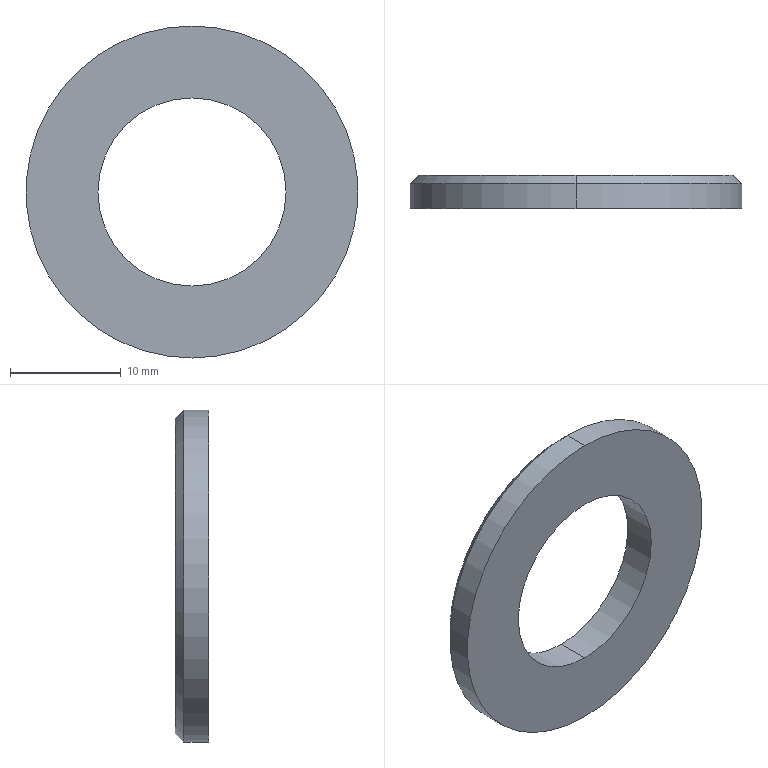Part | STEP file | Flat Washer GB/T97.2-1985 Chamfered Type Grade A 16x3 | 1 solid | 8 faces | box 30 x 3 x 30 mm | volume 1414 mm3 | cylinder 4 | cone 2 | plane 2 | commonest cylinder face diameters 17 x2 30 x2
STEP:
#1=CARTESIAN_POINT('',(0.,0.,0.));
#2=DIRECTION('',(0.,0.,1.));
#3=DIRECTION('',(1.,0.,0.));
#4=AXIS2_PLACEMENT_3D('',#1,#2,#3);
#5=CARTESIAN_POINT('',(0.,10.895,-15.));
#6=VERTEX_POINT('',#5);
#7=CARTESIAN_POINT('',(0.,10.895,15.));
#8=VERTEX_POINT('',#7);
#9=CARTESIAN_POINT('',(0.,10.895,0.));
#10=DIRECTION('',(0.,-1.,0.));
#11=DIRECTION('',(0.,0.,-1.));
#12=AXIS2_PLACEMENT_3D('',#9,#10,#11);
#13=CIRCLE('',#12,15.);
#14=CARTESIAN_POINT('',(0.,0.,0.));
#15=DIRECTION('',(0.,-1.,0.));
#16=DIRECTION('',(0.,0.,-1.));
#17=AXIS2_PLACEMENT_3D('',#14,#15,#16);
#18=CYLINDRICAL_SURFACE('',#17,15.);
#19=CARTESIAN_POINT('',(0.,-10.895));
#20=DIRECTION('',(1.,0.));
#21=VECTOR('',#20,1.);
#22=LINE('',#19,#21);
#23=(GEOMETRIC_REPRESENTATION_CONTEXT(2)PARAMETRIC_REPRESENTATION_CONTEXT()REPRESENTATION_CONTEXT('',''));
#24=DEFINITIONAL_REPRESENTATION('',(#22),#23);
#25=PCURVE('',#18,#24);
#26=CARTESIAN_POINT('',(0.,11.645,0.));
#27=DIRECTION('',(0.,-1.,0.));
#28=DIRECTION('',(0.,0.,-1.));
#29=AXIS2_PLACEMENT_3D('',#26,#27,#28);
#30=CONICAL_SURFACE('',#29,14.25,0.7854);
#31=CARTESIAN_POINT('',(0.,0.75));
#32=DIRECTION('',(1.,0.));
#33=VECTOR('',#32,1.);
#34=LINE('',#31,#33);
#35=(GEOMETRIC_REPRESENTATION_CONTEXT(2)PARAMETRIC_REPRESENTATION_CONTEXT()REPRESENTATION_CONTEXT('',''));
#36=DEFINITIONAL_REPRESENTATION('',(#34),#35);
#37=PCURVE('',#30,#36);
#38=SURFACE_CURVE('',#13,(#25,#37),.PCURVE_S1.);
#39=EDGE_CURVE('',#6,#8,#38,.T.);
#40=ORIENTED_EDGE('',*,*,#39,.T.);
#41=CARTESIAN_POINT('',(0.,8.645,15.));
#42=VERTEX_POINT('',#41);
#43=CARTESIAN_POINT('',(0.,0.,15.));
#44=DIRECTION('',(0.,-1.,0.));
#45=VECTOR('',#44,1.);
#46=LINE('',#43,#45);
#47=CARTESIAN_POINT('',(3.142,0.));
#48=DIRECTION('',(0.,1.));
#49=VECTOR('',#48,1.);
#50=LINE('',#47,#49);
#51=(GEOMETRIC_REPRESENTATION_CONTEXT(2)PARAMETRIC_REPRESENTATION_CONTEXT()REPRESENTATION_CONTEXT('',''));
#52=DEFINITIONAL_REPRESENTATION('',(#50),#51);
#53=PCURVE('',#18,#52);
#54=CARTESIAN_POINT('',(0.,0.,0.));
#55=DIRECTION('',(0.,-1.,0.));
#56=DIRECTION('',(0.,0.,-1.));
#57=AXIS2_PLACEMENT_3D('',#54,#55,#56);
#58=CYLINDRICAL_SURFACE('',#57,15.);
#59=CARTESIAN_POINT('',(3.142,0.));
#60=DIRECTION('',(0.,1.));
#61=VECTOR('',#60,1.);
#62=LINE('',#59,#61);
#63=(GEOMETRIC_REPRESENTATION_CONTEXT(2)PARAMETRIC_REPRESENTATION_CONTEXT()REPRESENTATION_CONTEXT('',''));
#64=DEFINITIONAL_REPRESENTATION('',(#62),#63);
#65=PCURVE('',#58,#64);
#66=SURFACE_CURVE('',#46,(#53,#65),.PCURVE_S1.);
#67=EDGE_CURVE('',#8,#42,#66,.T.);
#68=ORIENTED_EDGE('',*,*,#67,.T.);
#69=CARTESIAN_POINT('',(0.,8.645,-15.));
#70=VERTEX_POINT('',#69);
#71=CARTESIAN_POINT('',(0.,8.645,0.));
#72=DIRECTION('',(0.,-1.,0.));
#73=DIRECTION('',(0.,0.,-1.));
#74=AXIS2_PLACEMENT_3D('',#71,#72,#73);
#75=CIRCLE('',#74,15.);
#76=CARTESIAN_POINT('',(0.,-8.645));
#77=DIRECTION('',(1.,0.));
#78=VECTOR('',#77,1.);
#79=LINE('',#76,#78);
#80=(GEOMETRIC_REPRESENTATION_CONTEXT(2)PARAMETRIC_REPRESENTATION_CONTEXT()REPRESENTATION_CONTEXT('',''));
#81=DEFINITIONAL_REPRESENTATION('',(#79),#80);
#82=PCURVE('',#18,#81);
#83=CARTESIAN_POINT('',(-8.5,8.645,0.));
#84=DIRECTION('',(0.,1.,0.));
#85=DIRECTION('',(0.,0.,1.));
#86=AXIS2_PLACEMENT_3D('',#83,#84,#85);
#87=PLANE('',#86);
#88=CARTESIAN_POINT('',(-15.,8.5));
#89=CARTESIAN_POINT('',(-15.,34.481));
#90=CARTESIAN_POINT('',(7.5,21.49));
#91=CARTESIAN_POINT('',(30.,8.5));
#92=CARTESIAN_POINT('',(7.5,-4.49));
#93=CARTESIAN_POINT('',(-15.,-17.481));
#94=CARTESIAN_POINT('',(-15.,8.5));
#95=(BOUNDED_CURVE()B_SPLINE_CURVE(2,(#88,#89,#90,#91,#92,#93,#94),.UNSPECIFIED.,.T.,.F.)B_SPLINE_CURVE_WITH_KNOTS((1,2,2,2,2,1),(-2.094,0.,2.094,4.189,6.283,8.378),.UNSPECIFIED.)CURVE()GEOMETRIC_REPRESENTATION_ITEM()RATIONAL_B_SPLINE_CURVE((1.,0.5,1.,0.5,1.,0.5,1.))REPRESENTATION_ITEM(''));
#96=(GEOMETRIC_REPRESENTATION_CONTEXT(2)PARAMETRIC_REPRESENTATION_CONTEXT()REPRESENTATION_CONTEXT('',''));
#97=DEFINITIONAL_REPRESENTATION('',(#95),#96);
#98=PCURVE('',#87,#97);
#99=SURFACE_CURVE('',#75,(#82,#98),.PCURVE_S1.);
#100=EDGE_CURVE('',#70,#42,#99,.T.);
#101=ORIENTED_EDGE('',*,*,#100,.F.);
#102=CARTESIAN_POINT('',(0.,0.,-15.));
#103=DIRECTION('',(0.,-1.,0.));
#104=VECTOR('',#103,1.);
#105=LINE('',#102,#104);
#106=CARTESIAN_POINT('',(0.,0.));
#107=DIRECTION('',(0.,1.));
#108=VECTOR('',#107,1.);
#109=LINE('',#106,#108);
#110=(GEOMETRIC_REPRESENTATION_CONTEXT(2)PARAMETRIC_REPRESENTATION_CONTEXT()REPRESENTATION_CONTEXT('',''));
#111=DEFINITIONAL_REPRESENTATION('',(#109),#110);
#112=PCURVE('',#18,#111);
#113=CARTESIAN_POINT('',(6.283,0.));
#114=DIRECTION('',(0.,1.));
#115=VECTOR('',#114,1.);
#116=LINE('',#113,#115);
#117=(GEOMETRIC_REPRESENTATION_CONTEXT(2)PARAMETRIC_REPRESENTATION_CONTEXT()REPRESENTATION_CONTEXT('',''));
#118=DEFINITIONAL_REPRESENTATION('',(#116),#117);
#119=PCURVE('',#58,#118);
#120=SURFACE_CURVE('',#105,(#112,#119),.PCURVE_S1.);
#121=EDGE_CURVE('',#6,#70,#120,.T.);
#122=ORIENTED_EDGE('',*,*,#121,.F.);
#123=EDGE_LOOP('',(#40,#68,#101,#122));
#124=FACE_BOUND('',#123,.T.);
#125=ADVANCED_FACE('',(#124),#18,.T.);
#126=CARTESIAN_POINT('',(0.,11.645,-14.25));
#127=VERTEX_POINT('',#126);
#128=CARTESIAN_POINT('',(0.,11.645,14.25));
#129=VERTEX_POINT('',#128);
#130=CARTESIAN_POINT('',(0.,11.645,0.));
#131=DIRECTION('',(0.,-1.,0.));
#132=DIRECTION('',(0.,0.,-1.));
#133=AXIS2_PLACEMENT_3D('',#130,#131,#132);
#134=CIRCLE('',#133,14.25);
#135=CARTESIAN_POINT('',(0.,0.));
#136=DIRECTION('',(1.,0.));
#137=VECTOR('',#136,1.);
#138=LINE('',#135,#137);
#139=(GEOMETRIC_REPRESENTATION_CONTEXT(2)PARAMETRIC_REPRESENTATION_CONTEXT()REPRESENTATION_CONTEXT('',''));
#140=DEFINITIONAL_REPRESENTATION('',(#138),#139);
#141=PCURVE('',#30,#140);
#142=CARTESIAN_POINT('',(-8.5,11.645,0.));
#143=DIRECTION('',(0.,-1.,0.));
#144=DIRECTION('',(0.,0.,-1.));
#145=AXIS2_PLACEMENT_3D('',#142,#143,#144);
#146=PLANE('',#145);
#147=CARTESIAN_POINT('',(0.,8.5));
#148=DIRECTION('',(1.,0.));
#149=AXIS2_PLACEMENT_2D('',#147,#148);
#150=CIRCLE('',#149,14.25);
#151=(GEOMETRIC_REPRESENTATION_CONTEXT(2)PARAMETRIC_REPRESENTATION_CONTEXT()REPRESENTATION_CONTEXT('',''));
#152=DEFINITIONAL_REPRESENTATION('',(#150),#151);
#153=PCURVE('',#146,#152);
#154=SURFACE_CURVE('',#134,(#141,#153),.PCURVE_S1.);
#155=EDGE_CURVE('',#127,#129,#154,.T.);
#156=ORIENTED_EDGE('',*,*,#155,.T.);
#157=CARTESIAN_POINT('',(0.,11.645,14.25));
#158=DIRECTION('',(0.,-0.7071,0.7071));
#159=VECTOR('',#158,1.);
#160=LINE('',#157,#159);
#161=CARTESIAN_POINT('',(3.142,0.));
#162=DIRECTION('',(0.,1.));
#163=VECTOR('',#162,1.);
#164=LINE('',#161,#163);
#165=(GEOMETRIC_REPRESENTATION_CONTEXT(2)PARAMETRIC_REPRESENTATION_CONTEXT()REPRESENTATION_CONTEXT('',''));
#166=DEFINITIONAL_REPRESENTATION('',(#164),#165);
#167=PCURVE('',#30,#166);
#168=CARTESIAN_POINT('',(0.,11.645,0.));
#169=DIRECTION('',(0.,-1.,0.));
#170=DIRECTION('',(0.,0.,-1.));
#171=AXIS2_PLACEMENT_3D('',#168,#169,#170);
#172=CONICAL_SURFACE('',#171,14.25,0.7854);
#173=CARTESIAN_POINT('',(3.142,0.));
#174=DIRECTION('',(0.,1.));
#175=VECTOR('',#174,1.);
#176=LINE('',#173,#175);
#177=(GEOMETRIC_REPRESENTATION_CONTEXT(2)PARAMETRIC_REPRESENTATION_CONTEXT()REPRESENTATION_CONTEXT('',''));
#178=DEFINITIONAL_REPRESENTATION('',(#176),#177);
#179=PCURVE('',#172,#178);
#180=SURFACE_CURVE('',#160,(#167,#179),.PCURVE_S1.);
#181=EDGE_CURVE('',#129,#8,#180,.T.);
#182=ORIENTED_EDGE('',*,*,#181,.T.);
#183=ORIENTED_EDGE('',*,*,#39,.F.);
#184=CARTESIAN_POINT('',(0.,11.645,-14.25));
#185=DIRECTION('',(0.,-0.7071,-0.7071));
#186=VECTOR('',#185,1.);
#187=LINE('',#184,#186);
#188=CARTESIAN_POINT('',(0.,0.));
#189=DIRECTION('',(0.,1.));
#190=VECTOR('',#189,1.);
#191=LINE('',#188,#190);
#192=(GEOMETRIC_REPRESENTATION_CONTEXT(2)PARAMETRIC_REPRESENTATION_CONTEXT()REPRESENTATION_CONTEXT('',''));
#193=DEFINITIONAL_REPRESENTATION('',(#191),#192);
#194=PCURVE('',#30,#193);
#195=CARTESIAN_POINT('',(6.283,0.));
#196=DIRECTION('',(0.,1.));
#197=VECTOR('',#196,1.);
#198=LINE('',#195,#197);
#199=(GEOMETRIC_REPRESENTATION_CONTEXT(2)PARAMETRIC_REPRESENTATION_CONTEXT()REPRESENTATION_CONTEXT('',''));
#200=DEFINITIONAL_REPRESENTATION('',(#198),#199);
#201=PCURVE('',#172,#200);
#202=SURFACE_CURVE('',#187,(#194,#201),.PCURVE_S1.);
#203=EDGE_CURVE('',#127,#6,#202,.T.);
#204=ORIENTED_EDGE('',*,*,#203,.F.);
#205=EDGE_LOOP('',(#156,#182,#183,#204));
#206=FACE_BOUND('',#205,.T.);
#207=ADVANCED_FACE('',(#206),#30,.T.);
#208=CARTESIAN_POINT('',(0.,11.645,-8.5));
#209=VERTEX_POINT('',#208);
#210=CARTESIAN_POINT('',(0.,8.645,-8.5));
#211=VERTEX_POINT('',#210);
#212=CARTESIAN_POINT('',(0.,0.,-8.5));
#213=DIRECTION('',(0.,-1.,0.));
#214=VECTOR('',#213,1.);
#215=LINE('',#212,#214);
#216=CARTESIAN_POINT('',(0.,0.,0.));
#217=DIRECTION('',(0.,-1.,0.));
#218=DIRECTION('',(0.,0.,-1.));
#219=AXIS2_PLACEMENT_3D('',#216,#217,#218);
#220=CYLINDRICAL_SURFACE('',#219,8.5);
#221=CARTESIAN_POINT('',(6.283,0.));
#222=DIRECTION('',(0.,1.));
#223=VECTOR('',#222,1.);
#224=LINE('',#221,#223);
#225=(GEOMETRIC_REPRESENTATION_CONTEXT(2)PARAMETRIC_REPRESENTATION_CONTEXT()REPRESENTATION_CONTEXT('',''));
#226=DEFINITIONAL_REPRESENTATION('',(#224),#225);
#227=PCURVE('',#220,#226);
#228=CARTESIAN_POINT('',(0.,0.,0.));
#229=DIRECTION('',(0.,-1.,0.));
#230=DIRECTION('',(0.,0.,-1.));
#231=AXIS2_PLACEMENT_3D('',#228,#229,#230);
#232=CYLINDRICAL_SURFACE('',#231,8.5);
#233=CARTESIAN_POINT('',(0.,0.));
#234=DIRECTION('',(0.,1.));
#235=VECTOR('',#234,1.);
#236=LINE('',#233,#235);
#237=(GEOMETRIC_REPRESENTATION_CONTEXT(2)PARAMETRIC_REPRESENTATION_CONTEXT()REPRESENTATION_CONTEXT('',''));
#238=DEFINITIONAL_REPRESENTATION('',(#236),#237);
#239=PCURVE('',#232,#238);
#240=SURFACE_CURVE('',#215,(#227,#239),.PCURVE_S1.);
#241=EDGE_CURVE('',#209,#211,#240,.T.);
#242=ORIENTED_EDGE('',*,*,#241,.T.);
#243=CARTESIAN_POINT('',(0.,8.645,8.5));
#244=VERTEX_POINT('',#243);
#245=CARTESIAN_POINT('',(0.,8.645,0.));
#246=DIRECTION('',(0.,-1.,0.));
#247=DIRECTION('',(0.,0.,-1.));
#248=AXIS2_PLACEMENT_3D('',#245,#246,#247);
#249=CIRCLE('',#248,8.5);
#250=CARTESIAN_POINT('',(0.,-8.645));
#251=DIRECTION('',(1.,0.));
#252=VECTOR('',#251,1.);
#253=LINE('',#250,#252);
#254=(GEOMETRIC_REPRESENTATION_CONTEXT(2)PARAMETRIC_REPRESENTATION_CONTEXT()REPRESENTATION_CONTEXT('',''));
#255=DEFINITIONAL_REPRESENTATION('',(#253),#254);
#256=PCURVE('',#220,#255);
#257=CARTESIAN_POINT('',(-8.5,8.5));
#258=CARTESIAN_POINT('',(-8.5,23.222));
#259=CARTESIAN_POINT('',(4.25,15.861));
#260=CARTESIAN_POINT('',(17.,8.5));
#261=CARTESIAN_POINT('',(4.25,1.139));
#262=CARTESIAN_POINT('',(-8.5,-6.222));
#263=CARTESIAN_POINT('',(-8.5,8.5));
#264=(BOUNDED_CURVE()B_SPLINE_CURVE(2,(#257,#258,#259,#260,#261,#262,#263),.UNSPECIFIED.,.T.,.F.)B_SPLINE_CURVE_WITH_KNOTS((1,2,2,2,2,1),(-2.094,0.,2.094,4.189,6.283,8.378),.UNSPECIFIED.)CURVE()GEOMETRIC_REPRESENTATION_ITEM()RATIONAL_B_SPLINE_CURVE((1.,0.5,1.,0.5,1.,0.5,1.))REPRESENTATION_ITEM(''));
#265=(GEOMETRIC_REPRESENTATION_CONTEXT(2)PARAMETRIC_REPRESENTATION_CONTEXT()REPRESENTATION_CONTEXT('',''));
#266=DEFINITIONAL_REPRESENTATION('',(#264),#265);
#267=PCURVE('',#87,#266);
#268=SURFACE_CURVE('',#249,(#256,#267),.PCURVE_S1.);
#269=EDGE_CURVE('',#244,#211,#268,.T.);
#270=ORIENTED_EDGE('',*,*,#269,.F.);
#271=CARTESIAN_POINT('',(0.,11.645,8.5));
#272=VERTEX_POINT('',#271);
#273=CARTESIAN_POINT('',(0.,0.,8.5));
#274=DIRECTION('',(0.,-1.,0.));
#275=VECTOR('',#274,1.);
#276=LINE('',#273,#275);
#277=CARTESIAN_POINT('',(3.142,0.));
#278=DIRECTION('',(0.,1.));
#279=VECTOR('',#278,1.);
#280=LINE('',#277,#279);
#281=(GEOMETRIC_REPRESENTATION_CONTEXT(2)PARAMETRIC_REPRESENTATION_CONTEXT()REPRESENTATION_CONTEXT('',''));
#282=DEFINITIONAL_REPRESENTATION('',(#280),#281);
#283=PCURVE('',#220,#282);
#284=CARTESIAN_POINT('',(3.142,0.));
#285=DIRECTION('',(0.,1.));
#286=VECTOR('',#285,1.);
#287=LINE('',#284,#286);
#288=(GEOMETRIC_REPRESENTATION_CONTEXT(2)PARAMETRIC_REPRESENTATION_CONTEXT()REPRESENTATION_CONTEXT('',''));
#289=DEFINITIONAL_REPRESENTATION('',(#287),#288);
#290=PCURVE('',#232,#289);
#291=SURFACE_CURVE('',#276,(#283,#290),.PCURVE_S1.);
#292=EDGE_CURVE('',#272,#244,#291,.T.);
#293=ORIENTED_EDGE('',*,*,#292,.F.);
#294=CARTESIAN_POINT('',(0.,11.645,0.));
#295=DIRECTION('',(0.,-1.,0.));
#296=DIRECTION('',(0.,0.,-1.));
#297=AXIS2_PLACEMENT_3D('',#294,#295,#296);
#298=CIRCLE('',#297,8.5);
#299=CARTESIAN_POINT('',(0.,-11.645));
#300=DIRECTION('',(1.,0.));
#301=VECTOR('',#300,1.);
#302=LINE('',#299,#301);
#303=(GEOMETRIC_REPRESENTATION_CONTEXT(2)PARAMETRIC_REPRESENTATION_CONTEXT()REPRESENTATION_CONTEXT('',''));
#304=DEFINITIONAL_REPRESENTATION('',(#302),#303);
#305=PCURVE('',#220,#304);
#306=CARTESIAN_POINT('',(0.,8.5));
#307=DIRECTION('',(1.,0.));
#308=AXIS2_PLACEMENT_2D('',#306,#307);
#309=CIRCLE('',#308,8.5);
#310=(GEOMETRIC_REPRESENTATION_CONTEXT(2)PARAMETRIC_REPRESENTATION_CONTEXT()REPRESENTATION_CONTEXT('',''));
#311=DEFINITIONAL_REPRESENTATION('',(#309),#310);
#312=PCURVE('',#146,#311);
#313=SURFACE_CURVE('',#298,(#305,#312),.PCURVE_S1.);
#314=EDGE_CURVE('',#272,#209,#313,.T.);
#315=ORIENTED_EDGE('',*,*,#314,.T.);
#316=EDGE_LOOP('',(#242,#270,#293,#315));
#317=FACE_BOUND('',#316,.F.);
#318=ADVANCED_FACE('',(#317),#220,.F.);
#319=CARTESIAN_POINT('',(0.,8.645,0.));
#320=DIRECTION('',(0.,-1.,0.));
#321=DIRECTION('',(0.,0.,-1.));
#322=AXIS2_PLACEMENT_3D('',#319,#320,#321);
#323=CIRCLE('',#322,8.5);
#324=CARTESIAN_POINT('',(0.,-8.645));
#325=DIRECTION('',(1.,0.));
#326=VECTOR('',#325,1.);
#327=LINE('',#324,#326);
#328=(GEOMETRIC_REPRESENTATION_CONTEXT(2)PARAMETRIC_REPRESENTATION_CONTEXT()REPRESENTATION_CONTEXT('',''));
#329=DEFINITIONAL_REPRESENTATION('',(#327),#328);
#330=PCURVE('',#232,#329);
#331=CARTESIAN_POINT('',(-8.5,8.5));
#332=CARTESIAN_POINT('',(-8.5,23.222));
#333=CARTESIAN_POINT('',(4.25,15.861));
#334=CARTESIAN_POINT('',(17.,8.5));
#335=CARTESIAN_POINT('',(4.25,1.139));
#336=CARTESIAN_POINT('',(-8.5,-6.222));
#337=CARTESIAN_POINT('',(-8.5,8.5));
#338=(BOUNDED_CURVE()B_SPLINE_CURVE(2,(#331,#332,#333,#334,#335,#336,#337),.UNSPECIFIED.,.T.,.F.)B_SPLINE_CURVE_WITH_KNOTS((1,2,2,2,2,1),(-2.094,0.,2.094,4.189,6.283,8.378),.UNSPECIFIED.)CURVE()GEOMETRIC_REPRESENTATION_ITEM()RATIONAL_B_SPLINE_CURVE((1.,0.5,1.,0.5,1.,0.5,1.))REPRESENTATION_ITEM(''));
#339=(GEOMETRIC_REPRESENTATION_CONTEXT(2)PARAMETRIC_REPRESENTATION_CONTEXT()REPRESENTATION_CONTEXT('',''));
#340=DEFINITIONAL_REPRESENTATION('',(#338),#339);
#341=PCURVE('',#87,#340);
#342=SURFACE_CURVE('',#323,(#330,#341),.PCURVE_S1.);
#343=EDGE_CURVE('',#211,#244,#342,.T.);
#344=ORIENTED_EDGE('',*,*,#343,.F.);
#345=ORIENTED_EDGE('',*,*,#241,.F.);
#346=CARTESIAN_POINT('',(0.,11.645,0.));
#347=DIRECTION('',(0.,-1.,0.));
#348=DIRECTION('',(0.,0.,-1.));
#349=AXIS2_PLACEMENT_3D('',#346,#347,#348);
#350=CIRCLE('',#349,8.5);
#351=CARTESIAN_POINT('',(0.,-11.645));
#352=DIRECTION('',(1.,0.));
#353=VECTOR('',#352,1.);
#354=LINE('',#351,#353);
#355=(GEOMETRIC_REPRESENTATION_CONTEXT(2)PARAMETRIC_REPRESENTATION_CONTEXT()REPRESENTATION_CONTEXT('',''));
#356=DEFINITIONAL_REPRESENTATION('',(#354),#355);
#357=PCURVE('',#232,#356);
#358=CARTESIAN_POINT('',(0.,8.5));
#359=DIRECTION('',(1.,0.));
#360=AXIS2_PLACEMENT_2D('',#358,#359);
#361=CIRCLE('',#360,8.5);
#362=(GEOMETRIC_REPRESENTATION_CONTEXT(2)PARAMETRIC_REPRESENTATION_CONTEXT()REPRESENTATION_CONTEXT('',''));
#363=DEFINITIONAL_REPRESENTATION('',(#361),#362);
#364=PCURVE('',#146,#363);
#365=SURFACE_CURVE('',#350,(#357,#364),.PCURVE_S1.);
#366=EDGE_CURVE('',#209,#272,#365,.T.);
#367=ORIENTED_EDGE('',*,*,#366,.T.);
#368=ORIENTED_EDGE('',*,*,#292,.T.);
#369=EDGE_LOOP('',(#344,#345,#367,#368));
#370=FACE_BOUND('',#369,.F.);
#371=ADVANCED_FACE('',(#370),#232,.F.);
#372=ORIENTED_EDGE('',*,*,#155,.F.);
#373=CARTESIAN_POINT('',(0.,11.645,0.));
#374=DIRECTION('',(0.,-1.,0.));
#375=DIRECTION('',(0.,0.,-1.));
#376=AXIS2_PLACEMENT_3D('',#373,#374,#375);
#377=CIRCLE('',#376,14.25);
#378=CARTESIAN_POINT('',(0.,8.5));
#379=DIRECTION('',(1.,0.));
#380=AXIS2_PLACEMENT_2D('',#378,#379);
#381=CIRCLE('',#380,14.25);
#382=(GEOMETRIC_REPRESENTATION_CONTEXT(2)PARAMETRIC_REPRESENTATION_CONTEXT()REPRESENTATION_CONTEXT('',''));
#383=DEFINITIONAL_REPRESENTATION('',(#381),#382);
#384=PCURVE('',#146,#383);
#385=CARTESIAN_POINT('',(0.,0.));
#386=DIRECTION('',(1.,0.));
#387=VECTOR('',#386,1.);
#388=LINE('',#385,#387);
#389=(GEOMETRIC_REPRESENTATION_CONTEXT(2)PARAMETRIC_REPRESENTATION_CONTEXT()REPRESENTATION_CONTEXT('',''));
#390=DEFINITIONAL_REPRESENTATION('',(#388),#389);
#391=PCURVE('',#172,#390);
#392=SURFACE_CURVE('',#377,(#384,#391),.PCURVE_S1.);
#393=EDGE_CURVE('',#129,#127,#392,.T.);
#394=ORIENTED_EDGE('',*,*,#393,.F.);
#395=EDGE_LOOP('',(#372,#394));
#396=FACE_BOUND('',#395,.T.);
#397=ORIENTED_EDGE('',*,*,#366,.T.);
#398=ORIENTED_EDGE('',*,*,#314,.T.);
#399=EDGE_LOOP('',(#397,#398));
#400=FACE_BOUND('',#399,.T.);
#401=ADVANCED_FACE('',(#396,#400),#146,.F.);
#402=ORIENTED_EDGE('',*,*,#181,.F.);
#403=ORIENTED_EDGE('',*,*,#393,.T.);
#404=ORIENTED_EDGE('',*,*,#203,.T.);
#405=CARTESIAN_POINT('',(0.,10.895,0.));
#406=DIRECTION('',(0.,-1.,0.));
#407=DIRECTION('',(0.,0.,-1.));
#408=AXIS2_PLACEMENT_3D('',#405,#406,#407);
#409=CIRCLE('',#408,15.);
#410=CARTESIAN_POINT('',(0.,0.75));
#411=DIRECTION('',(1.,0.));
#412=VECTOR('',#411,1.);
#413=LINE('',#410,#412);
#414=(GEOMETRIC_REPRESENTATION_CONTEXT(2)PARAMETRIC_REPRESENTATION_CONTEXT()REPRESENTATION_CONTEXT('',''));
#415=DEFINITIONAL_REPRESENTATION('',(#413),#414);
#416=PCURVE('',#172,#415);
#417=CARTESIAN_POINT('',(0.,-10.895));
#418=DIRECTION('',(1.,0.));
#419=VECTOR('',#418,1.);
#420=LINE('',#417,#419);
#421=(GEOMETRIC_REPRESENTATION_CONTEXT(2)PARAMETRIC_REPRESENTATION_CONTEXT()REPRESENTATION_CONTEXT('',''));
#422=DEFINITIONAL_REPRESENTATION('',(#420),#421);
#423=PCURVE('',#58,#422);
#424=SURFACE_CURVE('',#409,(#416,#423),.PCURVE_S1.);
#425=EDGE_CURVE('',#8,#6,#424,.T.);
#426=ORIENTED_EDGE('',*,*,#425,.F.);
#427=EDGE_LOOP('',(#402,#403,#404,#426));
#428=FACE_BOUND('',#427,.T.);
#429=ADVANCED_FACE('',(#428),#172,.T.);
#430=ORIENTED_EDGE('',*,*,#67,.F.);
#431=ORIENTED_EDGE('',*,*,#425,.T.);
#432=ORIENTED_EDGE('',*,*,#121,.T.);
#433=CARTESIAN_POINT('',(0.,8.645,0.));
#434=DIRECTION('',(0.,-1.,0.));
#435=DIRECTION('',(0.,0.,-1.));
#436=AXIS2_PLACEMENT_3D('',#433,#434,#435);
#437=CIRCLE('',#436,15.);
#438=CARTESIAN_POINT('',(0.,-8.645));
#439=DIRECTION('',(1.,0.));
#440=VECTOR('',#439,1.);
#441=LINE('',#438,#440);
#442=(GEOMETRIC_REPRESENTATION_CONTEXT(2)PARAMETRIC_REPRESENTATION_CONTEXT()REPRESENTATION_CONTEXT('',''));
#443=DEFINITIONAL_REPRESENTATION('',(#441),#442);
#444=PCURVE('',#58,#443);
#445=CARTESIAN_POINT('',(-15.,8.5));
#446=CARTESIAN_POINT('',(-15.,34.481));
#447=CARTESIAN_POINT('',(7.5,21.49));
#448=CARTESIAN_POINT('',(30.,8.5));
#449=CARTESIAN_POINT('',(7.5,-4.49));
#450=CARTESIAN_POINT('',(-15.,-17.481));
#451=CARTESIAN_POINT('',(-15.,8.5));
#452=(BOUNDED_CURVE()B_SPLINE_CURVE(2,(#445,#446,#447,#448,#449,#450,#451),.UNSPECIFIED.,.T.,.F.)B_SPLINE_CURVE_WITH_KNOTS((1,2,2,2,2,1),(-2.094,0.,2.094,4.189,6.283,8.378),.UNSPECIFIED.)CURVE()GEOMETRIC_REPRESENTATION_ITEM()RATIONAL_B_SPLINE_CURVE((1.,0.5,1.,0.5,1.,0.5,1.))REPRESENTATION_ITEM(''));
#453=(GEOMETRIC_REPRESENTATION_CONTEXT(2)PARAMETRIC_REPRESENTATION_CONTEXT()REPRESENTATION_CONTEXT('',''));
#454=DEFINITIONAL_REPRESENTATION('',(#452),#453);
#455=PCURVE('',#87,#454);
#456=SURFACE_CURVE('',#437,(#444,#455),.PCURVE_S1.);
#457=EDGE_CURVE('',#42,#70,#456,.T.);
#458=ORIENTED_EDGE('',*,*,#457,.F.);
#459=EDGE_LOOP('',(#430,#431,#432,#458));
#460=FACE_BOUND('',#459,.T.);
#461=ADVANCED_FACE('',(#460),#58,.T.);
#462=ORIENTED_EDGE('',*,*,#343,.F.);
#463=ORIENTED_EDGE('',*,*,#269,.F.);
#464=EDGE_LOOP('',(#462,#463));
#465=FACE_BOUND('',#464,.T.);
#466=ORIENTED_EDGE('',*,*,#100,.T.);
#467=ORIENTED_EDGE('',*,*,#457,.T.);
#468=EDGE_LOOP('',(#466,#467));
#469=FACE_BOUND('',#468,.T.);
#470=ADVANCED_FACE('',(#465,#469),#87,.F.);
#471=CLOSED_SHELL('',(#125,#207,#318,#371,#401,#429,#461,#470));
#472=MANIFOLD_SOLID_BREP('',#471);
#473=(LENGTH_UNIT()NAMED_UNIT(*)SI_UNIT(.MILLI.,.METRE.));
#474=UNCERTAINTY_MEASURE_WITH_UNIT(LENGTH_MEASURE(0.0000001),#473,'','');
#475=(NAMED_UNIT(*)PLANE_ANGLE_UNIT()SI_UNIT($,.RADIAN.));
#476=(NAMED_UNIT(*)SI_UNIT($,.STERADIAN.)SOLID_ANGLE_UNIT());
#477=(GEOMETRIC_REPRESENTATION_CONTEXT(3)GLOBAL_UNCERTAINTY_ASSIGNED_CONTEXT((#474))GLOBAL_UNIT_ASSIGNED_CONTEXT((#473,#475,#476))REPRESENTATION_CONTEXT('',''));
#478=ADVANCED_BREP_SHAPE_REPRESENTATION('',(#4,#472),#477);